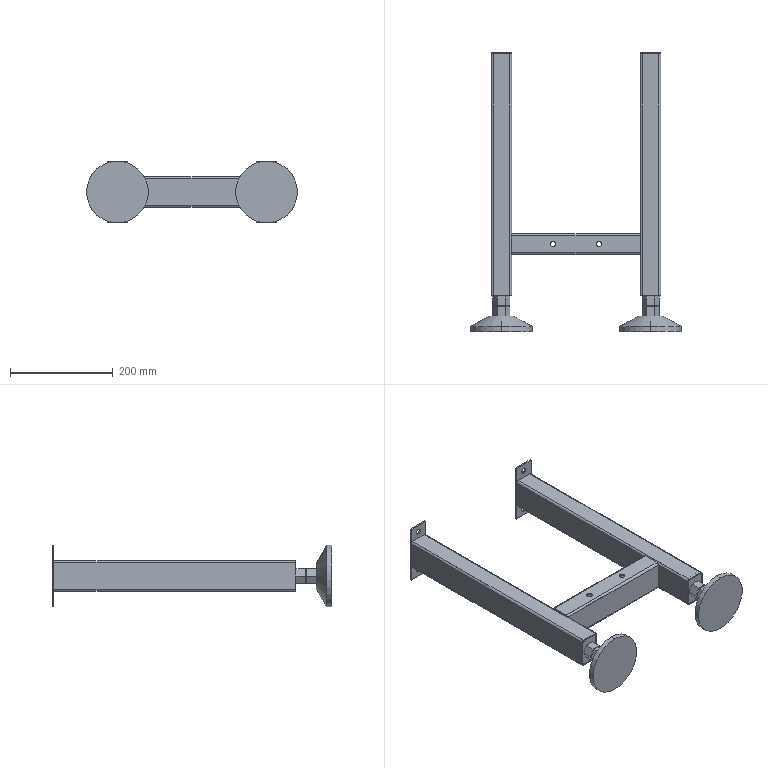Part | SolidWorks | features MoveCopyBody 4, Stock 4, ICE 3, WeldMemberFeat 2, HoleWzd 1, MirrorSolid 1, WeldCornerFeat 1, WeldmentFeature 1 | 15 solids | 274 faces | box 410 x 543 x 120 mm | volume 1073407 mm3 | plane 114 | cone 100 | cylinder 60 | commonest cylinder face diameters 10.5 x16 20 x16 4 x12 8 x12 17.5 x4